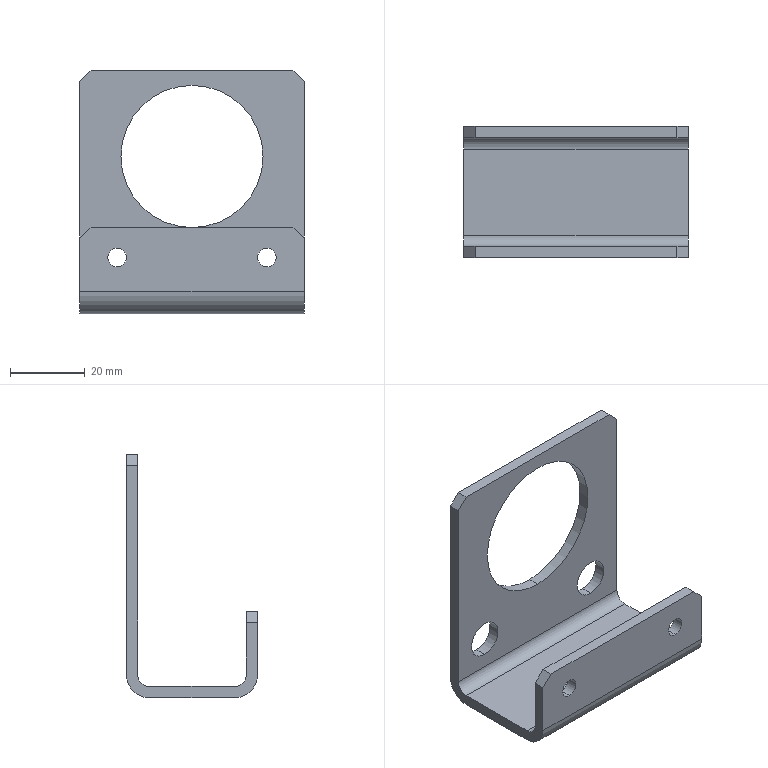Part | SolidWorks | features BaseBody 1 | 1 solid | 28 faces | box 60 x 35 x 65 mm | volume 16319 mm3 | cylinder 14 | plane 14 | commonest cylinder face diameters 5 x4 10 x4 6 x2 12 x2 38 x2
STEP:
#1=CARTESIAN_POINT('',(20.,29.,8.5));
#2=VERTEX_POINT('',#1);
#3=CARTESIAN_POINT('',(20.,29.,-1.5));
#4=VERTEX_POINT('',#3);
#5=CARTESIAN_POINT('',(20.,29.,3.5));
#6=DIRECTION('',(0.,-1.,0.));
#7=DIRECTION('',(0.,0.,-1.));
#8=AXIS2_PLACEMENT_3D('',#5,#6,#7);
#9=CIRCLE('',#8,5.);
#10=EDGE_CURVE('',#2,#4,#9,.T.);
#11=ORIENTED_EDGE('',*,*,#10,.T.);
#12=CARTESIAN_POINT('',(20.,32.,-1.5));
#13=VERTEX_POINT('',#12);
#14=CARTESIAN_POINT('',(20.,22.,-1.5));
#15=DIRECTION('',(0.,1.,0.));
#16=VECTOR('',#15,1000.);
#17=LINE('',#14,#16);
#18=EDGE_CURVE('',#4,#13,#17,.T.);
#19=ORIENTED_EDGE('',*,*,#18,.T.);
#20=CARTESIAN_POINT('',(20.,32.,8.5));
#21=VERTEX_POINT('',#20);
#22=CARTESIAN_POINT('',(20.,32.,3.5));
#23=DIRECTION('',(0.,1.,0.));
#24=DIRECTION('',(0.,0.,1.));
#25=AXIS2_PLACEMENT_3D('',#22,#23,#24);
#26=CIRCLE('',#25,5.);
#27=EDGE_CURVE('',#13,#21,#26,.T.);
#28=ORIENTED_EDGE('',*,*,#27,.T.);
#29=CARTESIAN_POINT('',(20.,22.,8.5));
#30=DIRECTION('',(0.,1.,0.));
#31=VECTOR('',#30,1000.);
#32=LINE('',#29,#31);
#33=EDGE_CURVE('',#2,#21,#32,.T.);
#34=ORIENTED_EDGE('',*,*,#33,.F.);
#35=EDGE_LOOP('',(#11,#19,#28,#34));
#36=FACE_OUTER_BOUND('',#35,.T.);
#37=CARTESIAN_POINT('',(20.,22.,3.5));
#38=DIRECTION('',(0.,1.,0.));
#39=DIRECTION('',(0.,0.,1.));
#40=AXIS2_PLACEMENT_3D('',#37,#38,#39);
#41=CYLINDRICAL_SURFACE('',#40,5.);
#42=ADVANCED_FACE('',(#36),#41,.F.);
#43=CARTESIAN_POINT('',(-20.,29.,8.5));
#44=VERTEX_POINT('',#43);
#45=CARTESIAN_POINT('',(-20.,29.,-1.5));
#46=VERTEX_POINT('',#45);
#47=CARTESIAN_POINT('',(-20.,29.,3.5));
#48=DIRECTION('',(0.,-1.,0.));
#49=DIRECTION('',(0.,0.,-1.));
#50=AXIS2_PLACEMENT_3D('',#47,#48,#49);
#51=CIRCLE('',#50,5.);
#52=EDGE_CURVE('',#44,#46,#51,.T.);
#53=ORIENTED_EDGE('',*,*,#52,.T.);
#54=CARTESIAN_POINT('',(-20.,32.,-1.5));
#55=VERTEX_POINT('',#54);
#56=CARTESIAN_POINT('',(-20.,22.,-1.5));
#57=DIRECTION('',(0.,1.,0.));
#58=VECTOR('',#57,1000.);
#59=LINE('',#56,#58);
#60=EDGE_CURVE('',#46,#55,#59,.T.);
#61=ORIENTED_EDGE('',*,*,#60,.T.);
#62=CARTESIAN_POINT('',(-20.,32.,8.5));
#63=VERTEX_POINT('',#62);
#64=CARTESIAN_POINT('',(-20.,32.,3.5));
#65=DIRECTION('',(0.,1.,0.));
#66=DIRECTION('',(0.,0.,1.));
#67=AXIS2_PLACEMENT_3D('',#64,#65,#66);
#68=CIRCLE('',#67,5.);
#69=EDGE_CURVE('',#55,#63,#68,.T.);
#70=ORIENTED_EDGE('',*,*,#69,.T.);
#71=CARTESIAN_POINT('',(-20.,22.,8.5));
#72=DIRECTION('',(0.,1.,0.));
#73=VECTOR('',#72,1000.);
#74=LINE('',#71,#73);
#75=EDGE_CURVE('',#44,#63,#74,.T.);
#76=ORIENTED_EDGE('',*,*,#75,.F.);
#77=EDGE_LOOP('',(#53,#61,#70,#76));
#78=FACE_OUTER_BOUND('',#77,.T.);
#79=CARTESIAN_POINT('',(-20.,22.,3.5));
#80=DIRECTION('',(0.,1.,0.));
#81=DIRECTION('',(0.,0.,1.));
#82=AXIS2_PLACEMENT_3D('',#79,#80,#81);
#83=CYLINDRICAL_SURFACE('',#82,5.);
#84=ADVANCED_FACE('',(#78),#83,.F.);
#85=CARTESIAN_POINT('',(0.,29.,11.5));
#86=VERTEX_POINT('',#85);
#87=CARTESIAN_POINT('',(0.,29.,49.5));
#88=VERTEX_POINT('',#87);
#89=CARTESIAN_POINT('',(0.,29.,30.5));
#90=DIRECTION('',(0.,1.,0.));
#91=DIRECTION('',(0.,0.,-1.));
#92=AXIS2_PLACEMENT_3D('',#89,#90,#91);
#93=CIRCLE('',#92,19.);
#94=EDGE_CURVE('',#86,#88,#93,.T.);
#95=ORIENTED_EDGE('',*,*,#94,.F.);
#96=CARTESIAN_POINT('',(0.,32.,11.5));
#97=VERTEX_POINT('',#96);
#98=CARTESIAN_POINT('',(0.,-3.001,11.5));
#99=DIRECTION('',(0.,1.,0.));
#100=VECTOR('',#99,1000.);
#101=LINE('',#98,#100);
#102=EDGE_CURVE('',#86,#97,#101,.T.);
#103=ORIENTED_EDGE('',*,*,#102,.T.);
#104=CARTESIAN_POINT('',(0.,32.,49.5));
#105=VERTEX_POINT('',#104);
#106=CARTESIAN_POINT('',(0.,32.,30.5));
#107=DIRECTION('',(0.,1.,0.));
#108=DIRECTION('',(0.,0.,1.));
#109=AXIS2_PLACEMENT_3D('',#106,#107,#108);
#110=CIRCLE('',#109,19.);
#111=EDGE_CURVE('',#97,#105,#110,.T.);
#112=ORIENTED_EDGE('',*,*,#111,.T.);
#113=CARTESIAN_POINT('',(0.,-3.001,49.5));
#114=DIRECTION('',(0.,1.,0.));
#115=VECTOR('',#114,1000.);
#116=LINE('',#113,#115);
#117=EDGE_CURVE('',#88,#105,#116,.T.);
#118=ORIENTED_EDGE('',*,*,#117,.F.);
#119=EDGE_LOOP('',(#95,#103,#112,#118));
#120=FACE_OUTER_BOUND('',#119,.T.);
#121=CARTESIAN_POINT('',(0.,-3.001,30.5));
#122=DIRECTION('',(0.,1.,0.));
#123=DIRECTION('',(0.,0.,1.));
#124=AXIS2_PLACEMENT_3D('',#121,#122,#123);
#125=CYLINDRICAL_SURFACE('',#124,19.);
#126=ADVANCED_FACE('',(#120),#125,.F.);
#127=CARTESIAN_POINT('',(-20.,0.,1.));
#128=VERTEX_POINT('',#127);
#129=CARTESIAN_POINT('',(-20.,0.,6.));
#130=VERTEX_POINT('',#129);
#131=CARTESIAN_POINT('',(-20.,0.,3.5));
#132=DIRECTION('',(0.,1.,0.));
#133=DIRECTION('',(0.,0.,1.));
#134=AXIS2_PLACEMENT_3D('',#131,#132,#133);
#135=CIRCLE('',#134,2.5);
#136=EDGE_CURVE('',#128,#130,#135,.T.);
#137=ORIENTED_EDGE('',*,*,#136,.T.);
#138=CARTESIAN_POINT('',(-20.,-3.,6.));
#139=VERTEX_POINT('',#138);
#140=CARTESIAN_POINT('',(-20.,-3.,6.));
#141=DIRECTION('',(0.,-1.,0.));
#142=VECTOR('',#141,1000.);
#143=LINE('',#140,#142);
#144=EDGE_CURVE('',#130,#139,#143,.T.);
#145=ORIENTED_EDGE('',*,*,#144,.T.);
#146=CARTESIAN_POINT('',(-20.,-3.,1.));
#147=VERTEX_POINT('',#146);
#148=CARTESIAN_POINT('',(-20.,-3.,3.5));
#149=DIRECTION('',(0.,-1.,0.));
#150=DIRECTION('',(0.,0.,-1.));
#151=AXIS2_PLACEMENT_3D('',#148,#149,#150);
#152=CIRCLE('',#151,2.5);
#153=EDGE_CURVE('',#139,#147,#152,.T.);
#154=ORIENTED_EDGE('',*,*,#153,.T.);
#155=CARTESIAN_POINT('',(-20.,-3.,1.));
#156=DIRECTION('',(0.,-1.,0.));
#157=VECTOR('',#156,1000.);
#158=LINE('',#155,#157);
#159=EDGE_CURVE('',#128,#147,#158,.T.);
#160=ORIENTED_EDGE('',*,*,#159,.F.);
#161=EDGE_LOOP('',(#137,#145,#154,#160));
#162=FACE_OUTER_BOUND('',#161,.T.);
#163=CARTESIAN_POINT('',(-20.,-3.,3.5));
#164=DIRECTION('',(0.,-1.,0.));
#165=DIRECTION('',(0.,0.,-1.));
#166=AXIS2_PLACEMENT_3D('',#163,#164,#165);
#167=CYLINDRICAL_SURFACE('',#166,2.5);
#168=ADVANCED_FACE('',(#162),#167,.F.);
#169=CARTESIAN_POINT('',(20.,0.,1.));
#170=VERTEX_POINT('',#169);
#171=CARTESIAN_POINT('',(20.,0.,6.));
#172=VERTEX_POINT('',#171);
#173=CARTESIAN_POINT('',(20.,0.,3.5));
#174=DIRECTION('',(0.,1.,0.));
#175=DIRECTION('',(0.,0.,1.));
#176=AXIS2_PLACEMENT_3D('',#173,#174,#175);
#177=CIRCLE('',#176,2.5);
#178=EDGE_CURVE('',#170,#172,#177,.T.);
#179=ORIENTED_EDGE('',*,*,#178,.T.);
#180=CARTESIAN_POINT('',(20.,-3.,6.));
#181=VERTEX_POINT('',#180);
#182=CARTESIAN_POINT('',(20.,-3.,6.));
#183=DIRECTION('',(0.,-1.,0.));
#184=VECTOR('',#183,1000.);
#185=LINE('',#182,#184);
#186=EDGE_CURVE('',#172,#181,#185,.T.);
#187=ORIENTED_EDGE('',*,*,#186,.T.);
#188=CARTESIAN_POINT('',(20.,-3.,1.));
#189=VERTEX_POINT('',#188);
#190=CARTESIAN_POINT('',(20.,-3.,3.5));
#191=DIRECTION('',(0.,-1.,0.));
#192=DIRECTION('',(0.,0.,-1.));
#193=AXIS2_PLACEMENT_3D('',#190,#191,#192);
#194=CIRCLE('',#193,2.5);
#195=EDGE_CURVE('',#181,#189,#194,.T.);
#196=ORIENTED_EDGE('',*,*,#195,.T.);
#197=CARTESIAN_POINT('',(20.,-3.,1.));
#198=DIRECTION('',(0.,-1.,0.));
#199=VECTOR('',#198,1000.);
#200=LINE('',#197,#199);
#201=EDGE_CURVE('',#170,#189,#200,.T.);
#202=ORIENTED_EDGE('',*,*,#201,.F.);
#203=EDGE_LOOP('',(#179,#187,#196,#202));
#204=FACE_OUTER_BOUND('',#203,.T.);
#205=CARTESIAN_POINT('',(20.,-3.,3.5));
#206=DIRECTION('',(0.,-1.,0.));
#207=DIRECTION('',(0.,0.,-1.));
#208=AXIS2_PLACEMENT_3D('',#205,#206,#207);
#209=CYLINDRICAL_SURFACE('',#208,2.5);
#210=ADVANCED_FACE('',(#204),#209,.F.);
#211=CARTESIAN_POINT('',(27.,32.,53.5));
#212=VERTEX_POINT('',#211);
#213=CARTESIAN_POINT('',(30.,32.,50.5));
#214=VERTEX_POINT('',#213);
#215=CARTESIAN_POINT('',(30.,32.,50.5));
#216=DIRECTION('',(0.7071,0.,-0.7071));
#217=VECTOR('',#216,1000.);
#218=LINE('',#215,#217);
#219=EDGE_CURVE('',#212,#214,#218,.T.);
#220=ORIENTED_EDGE('',*,*,#219,.F.);
#221=CARTESIAN_POINT('',(27.,29.,53.5));
#222=VERTEX_POINT('',#221);
#223=CARTESIAN_POINT('',(27.,32.,53.5));
#224=DIRECTION('',(0.,1.,0.));
#225=VECTOR('',#224,1000.);
#226=LINE('',#223,#225);
#227=EDGE_CURVE('',#222,#212,#226,.T.);
#228=ORIENTED_EDGE('',*,*,#227,.F.);
#229=CARTESIAN_POINT('',(30.,29.,50.5));
#230=VERTEX_POINT('',#229);
#231=CARTESIAN_POINT('',(40.25,29.,40.25));
#232=DIRECTION('',(-0.7071,0.,0.7071));
#233=VECTOR('',#232,1000.);
#234=LINE('',#231,#233);
#235=EDGE_CURVE('',#230,#222,#234,.T.);
#236=ORIENTED_EDGE('',*,*,#235,.F.);
#237=CARTESIAN_POINT('',(30.,32.,50.5));
#238=DIRECTION('',(0.,-1.,0.));
#239=VECTOR('',#238,1000.);
#240=LINE('',#237,#239);
#241=EDGE_CURVE('',#214,#230,#240,.T.);
#242=ORIENTED_EDGE('',*,*,#241,.F.);
#243=EDGE_LOOP('',(#220,#228,#236,#242));
#244=FACE_OUTER_BOUND('',#243,.T.);
#245=CARTESIAN_POINT('',(30.,32.,50.5));
#246=DIRECTION('',(-0.7071,0.,-0.7071));
#247=DIRECTION('',(-0.7071,0.,0.7071));
#248=AXIS2_PLACEMENT_3D('',#245,#246,#247);
#249=PLANE('',#248);
#250=ADVANCED_FACE('',(#244),#249,.F.);
#251=CARTESIAN_POINT('',(-30.,32.,50.5));
#252=VERTEX_POINT('',#251);
#253=CARTESIAN_POINT('',(-27.,32.,53.5));
#254=VERTEX_POINT('',#253);
#255=CARTESIAN_POINT('',(-27.,32.,53.5));
#256=DIRECTION('',(0.7071,0.,0.7071));
#257=VECTOR('',#256,1000.);
#258=LINE('',#255,#257);
#259=EDGE_CURVE('',#252,#254,#258,.T.);
#260=ORIENTED_EDGE('',*,*,#259,.F.);
#261=CARTESIAN_POINT('',(-30.,29.,50.5));
#262=VERTEX_POINT('',#261);
#263=CARTESIAN_POINT('',(-30.,32.,50.5));
#264=DIRECTION('',(0.,1.,0.));
#265=VECTOR('',#264,1000.);
#266=LINE('',#263,#265);
#267=EDGE_CURVE('',#262,#252,#266,.T.);
#268=ORIENTED_EDGE('',*,*,#267,.F.);
#269=CARTESIAN_POINT('',(-27.,29.,53.5));
#270=VERTEX_POINT('',#269);
#271=CARTESIAN_POINT('',(-40.25,29.,40.25));
#272=DIRECTION('',(-0.7071,0.,-0.7071));
#273=VECTOR('',#272,1000.);
#274=LINE('',#271,#273);
#275=EDGE_CURVE('',#270,#262,#274,.T.);
#276=ORIENTED_EDGE('',*,*,#275,.F.);
#277=CARTESIAN_POINT('',(-27.,32.,53.5));
#278=DIRECTION('',(0.,-1.,0.));
#279=VECTOR('',#278,1000.);
#280=LINE('',#277,#279);
#281=EDGE_CURVE('',#254,#270,#280,.T.);
#282=ORIENTED_EDGE('',*,*,#281,.F.);
#283=EDGE_LOOP('',(#260,#268,#276,#282));
#284=FACE_OUTER_BOUND('',#283,.T.);
#285=CARTESIAN_POINT('',(-27.,32.,53.5));
#286=DIRECTION('',(0.7071,0.,-0.7071));
#287=DIRECTION('',(0.,-1.,0.));
#288=AXIS2_PLACEMENT_3D('',#285,#286,#287);
#289=PLANE('',#288);
#290=ADVANCED_FACE('',(#284),#289,.F.);
#291=CARTESIAN_POINT('',(-27.,-3.,11.5));
#292=VERTEX_POINT('',#291);
#293=CARTESIAN_POINT('',(-30.,-3.,8.5));
#294=VERTEX_POINT('',#293);
#295=CARTESIAN_POINT('',(-30.,-3.,8.5));
#296=DIRECTION('',(-0.7071,0.,-0.7071));
#297=VECTOR('',#296,1000.);
#298=LINE('',#295,#297);
#299=EDGE_CURVE('',#292,#294,#298,.T.);
#300=ORIENTED_EDGE('',*,*,#299,.F.);
#301=CARTESIAN_POINT('',(-27.,0.,11.5));
#302=VERTEX_POINT('',#301);
#303=CARTESIAN_POINT('',(-27.,-3.,11.5));
#304=DIRECTION('',(0.,-1.,0.));
#305=VECTOR('',#304,1000.);
#306=LINE('',#303,#305);
#307=EDGE_CURVE('',#302,#292,#306,.T.);
#308=ORIENTED_EDGE('',*,*,#307,.F.);
#309=CARTESIAN_POINT('',(-30.,0.,8.5));
#310=VERTEX_POINT('',#309);
#311=CARTESIAN_POINT('',(-19.25,0.,19.25));
#312=DIRECTION('',(0.7071,0.,0.7071));
#313=VECTOR('',#312,1000.);
#314=LINE('',#311,#313);
#315=EDGE_CURVE('',#310,#302,#314,.T.);
#316=ORIENTED_EDGE('',*,*,#315,.F.);
#317=CARTESIAN_POINT('',(-30.,-3.,8.5));
#318=DIRECTION('',(0.,1.,0.));
#319=VECTOR('',#318,1000.);
#320=LINE('',#317,#319);
#321=EDGE_CURVE('',#294,#310,#320,.T.);
#322=ORIENTED_EDGE('',*,*,#321,.F.);
#323=EDGE_LOOP('',(#300,#308,#316,#322));
#324=FACE_OUTER_BOUND('',#323,.T.);
#325=CARTESIAN_POINT('',(-30.,-3.,8.5));
#326=DIRECTION('',(0.7071,0.,-0.7071));
#327=DIRECTION('',(0.,-1.,0.));
#328=AXIS2_PLACEMENT_3D('',#325,#326,#327);
#329=PLANE('',#328);
#330=ADVANCED_FACE('',(#324),#329,.F.);
#331=CARTESIAN_POINT('',(30.,-3.,8.5));
#332=VERTEX_POINT('',#331);
#333=CARTESIAN_POINT('',(27.,-3.,11.5));
#334=VERTEX_POINT('',#333);
#335=CARTESIAN_POINT('',(27.,-3.,11.5));
#336=DIRECTION('',(-0.7071,0.,0.7071));
#337=VECTOR('',#336,1000.);
#338=LINE('',#335,#337);
#339=EDGE_CURVE('',#332,#334,#338,.T.);
#340=ORIENTED_EDGE('',*,*,#339,.F.);
#341=CARTESIAN_POINT('',(30.,0.,8.5));
#342=VERTEX_POINT('',#341);
#343=CARTESIAN_POINT('',(30.,-3.,8.5));
#344=DIRECTION('',(0.,-1.,0.));
#345=VECTOR('',#344,1000.);
#346=LINE('',#343,#345);
#347=EDGE_CURVE('',#342,#332,#346,.T.);
#348=ORIENTED_EDGE('',*,*,#347,.F.);
#349=CARTESIAN_POINT('',(27.,0.,11.5));
#350=VERTEX_POINT('',#349);
#351=CARTESIAN_POINT('',(19.25,0.,19.25));
#352=DIRECTION('',(0.7071,0.,-0.7071));
#353=VECTOR('',#352,1000.);
#354=LINE('',#351,#353);
#355=EDGE_CURVE('',#350,#342,#354,.T.);
#356=ORIENTED_EDGE('',*,*,#355,.F.);
#357=CARTESIAN_POINT('',(27.,-3.,11.5));
#358=DIRECTION('',(0.,1.,0.));
#359=VECTOR('',#358,1000.);
#360=LINE('',#357,#359);
#361=EDGE_CURVE('',#334,#350,#360,.T.);
#362=ORIENTED_EDGE('',*,*,#361,.F.);
#363=EDGE_LOOP('',(#340,#348,#356,#362));
#364=FACE_OUTER_BOUND('',#363,.T.);
#365=CARTESIAN_POINT('',(27.,-3.,11.5));
#366=DIRECTION('',(-0.7071,0.,-0.7071));
#367=DIRECTION('',(-0.7071,0.,0.7071));
#368=AXIS2_PLACEMENT_3D('',#365,#366,#367);
#369=PLANE('',#368);
#370=ADVANCED_FACE('',(#364),#369,.F.);
#371=CARTESIAN_POINT('',(0.,32.,53.5));
#372=DIRECTION('',(1.,0.,0.));
#373=VECTOR('',#372,1000.);
#374=LINE('',#371,#373);
#375=EDGE_CURVE('',#254,#212,#374,.T.);
#376=ORIENTED_EDGE('',*,*,#375,.F.);
#377=ORIENTED_EDGE('',*,*,#281,.T.);
#378=CARTESIAN_POINT('',(30.,29.,53.5));
#379=DIRECTION('',(1.,0.,0.));
#380=VECTOR('',#379,1000.);
#381=LINE('',#378,#380);
#382=EDGE_CURVE('',#270,#222,#381,.T.);
#383=ORIENTED_EDGE('',*,*,#382,.T.);
#384=ORIENTED_EDGE('',*,*,#227,.T.);
#385=EDGE_LOOP('',(#376,#377,#383,#384));
#386=FACE_OUTER_BOUND('',#385,.T.);
#387=CARTESIAN_POINT('',(30.,32.,53.5));
#388=DIRECTION('',(0.,0.,-1.));
#389=DIRECTION('',(0.,-1.,0.));
#390=AXIS2_PLACEMENT_3D('',#387,#388,#389);
#391=PLANE('',#390);
#392=ADVANCED_FACE('',(#386),#391,.F.);
#393=CARTESIAN_POINT('',(0.,29.,30.5));
#394=DIRECTION('',(0.,1.,0.));
#395=DIRECTION('',(0.,0.,-1.));
#396=AXIS2_PLACEMENT_3D('',#393,#394,#395);
#397=CIRCLE('',#396,19.);
#398=EDGE_CURVE('',#88,#86,#397,.T.);
#399=ORIENTED_EDGE('',*,*,#398,.T.);
#400=ORIENTED_EDGE('',*,*,#94,.T.);
#401=EDGE_LOOP('',(#399,#400));
#402=FACE_BOUND('',#401,.T.);
#403=ORIENTED_EDGE('',*,*,#52,.F.);
#404=CARTESIAN_POINT('',(-20.,29.,3.5));
#405=DIRECTION('',(0.,-1.,0.));
#406=DIRECTION('',(0.,0.,-1.));
#407=AXIS2_PLACEMENT_3D('',#404,#405,#406);
#408=CIRCLE('',#407,5.);
#409=EDGE_CURVE('',#46,#44,#408,.T.);
#410=ORIENTED_EDGE('',*,*,#409,.F.);
#411=EDGE_LOOP('',(#403,#410));
#412=FACE_BOUND('',#411,.T.);
#413=ORIENTED_EDGE('',*,*,#10,.F.);
#414=CARTESIAN_POINT('',(20.,29.,3.5));
#415=DIRECTION('',(0.,-1.,0.));
#416=DIRECTION('',(0.,0.,-1.));
#417=AXIS2_PLACEMENT_3D('',#414,#415,#416);
#418=CIRCLE('',#417,5.);
#419=EDGE_CURVE('',#4,#2,#418,.T.);
#420=ORIENTED_EDGE('',*,*,#419,.F.);
#421=EDGE_LOOP('',(#413,#420));
#422=FACE_BOUND('',#421,.T.);
#423=ORIENTED_EDGE('',*,*,#382,.F.);
#424=ORIENTED_EDGE('',*,*,#275,.T.);
#425=CARTESIAN_POINT('',(-30.,29.,-5.5));
#426=VERTEX_POINT('',#425);
#427=CARTESIAN_POINT('',(-30.,29.,53.5));
#428=DIRECTION('',(0.,0.,1.));
#429=VECTOR('',#428,1000.);
#430=LINE('',#427,#429);
#431=EDGE_CURVE('',#426,#262,#430,.T.);
#432=ORIENTED_EDGE('',*,*,#431,.F.);
#433=CARTESIAN_POINT('',(30.,29.,-5.5));
#434=VERTEX_POINT('',#433);
#435=CARTESIAN_POINT('',(30.,29.,-5.5));
#436=DIRECTION('',(-1.,0.,0.));
#437=VECTOR('',#436,1000.);
#438=LINE('',#435,#437);
#439=EDGE_CURVE('',#434,#426,#438,.T.);
#440=ORIENTED_EDGE('',*,*,#439,.F.);
#441=CARTESIAN_POINT('',(30.,29.,-8.5));
#442=DIRECTION('',(0.,0.,-1.));
#443=VECTOR('',#442,1000.);
#444=LINE('',#441,#443);
#445=EDGE_CURVE('',#230,#434,#444,.T.);
#446=ORIENTED_EDGE('',*,*,#445,.F.);
#447=ORIENTED_EDGE('',*,*,#235,.T.);
#448=EDGE_LOOP('',(#423,#424,#432,#440,#446,#447));
#449=FACE_OUTER_BOUND('',#448,.T.);
#450=CARTESIAN_POINT('',(0.,29.,0.));
#451=DIRECTION('',(0.,-1.,0.));
#452=DIRECTION('',(-1.,0.,0.));
#453=AXIS2_PLACEMENT_3D('',#450,#451,#452);
#454=PLANE('',#453);
#455=ADVANCED_FACE('',(#402,#412,#422,#449),#454,.T.);
#456=CARTESIAN_POINT('',(0.,32.,30.5));
#457=DIRECTION('',(0.,1.,0.));
#458=DIRECTION('',(0.,0.,1.));
#459=AXIS2_PLACEMENT_3D('',#456,#457,#458);
#460=CIRCLE('',#459,19.);
#461=EDGE_CURVE('',#105,#97,#460,.T.);
#462=ORIENTED_EDGE('',*,*,#461,.F.);
#463=ORIENTED_EDGE('',*,*,#111,.F.);
#464=EDGE_LOOP('',(#462,#463));
#465=FACE_BOUND('',#464,.T.);
#466=CARTESIAN_POINT('',(-20.,32.,3.5));
#467=DIRECTION('',(0.,1.,0.));
#468=DIRECTION('',(0.,0.,1.));
#469=AXIS2_PLACEMENT_3D('',#466,#467,#468);
#470=CIRCLE('',#469,5.);
#471=EDGE_CURVE('',#63,#55,#470,.T.);
#472=ORIENTED_EDGE('',*,*,#471,.F.);
#473=ORIENTED_EDGE('',*,*,#69,.F.);
#474=EDGE_LOOP('',(#472,#473));
#475=FACE_BOUND('',#474,.T.);
#476=CARTESIAN_POINT('',(20.,32.,3.5));
#477=DIRECTION('',(0.,1.,0.));
#478=DIRECTION('',(0.,0.,1.));
#479=AXIS2_PLACEMENT_3D('',#476,#477,#478);
#480=CIRCLE('',#479,5.);
#481=EDGE_CURVE('',#21,#13,#480,.T.);
#482=ORIENTED_EDGE('',*,*,#481,.F.);
#483=ORIENTED_EDGE('',*,*,#27,.F.);
#484=EDGE_LOOP('',(#482,#483));
#485=FACE_BOUND('',#484,.T.);
#486=CARTESIAN_POINT('',(-30.,32.,-5.5));
#487=VERTEX_POINT('',#486);
#488=CARTESIAN_POINT('',(-30.,32.,0.));
#489=DIRECTION('',(0.,0.,1.));
#490=VECTOR('',#489,1000.);
#491=LINE('',#488,#490);
#492=EDGE_CURVE('',#487,#252,#491,.T.);
#493=ORIENTED_EDGE('',*,*,#492,.T.);
#494=ORIENTED_EDGE('',*,*,#259,.T.);
#495=ORIENTED_EDGE('',*,*,#375,.T.);
#496=ORIENTED_EDGE('',*,*,#219,.T.);
#497=CARTESIAN_POINT('',(30.,32.,-5.5));
#498=VERTEX_POINT('',#497);
#499=CARTESIAN_POINT('',(30.,32.,0.));
#500=DIRECTION('',(0.,0.,-1.));
#501=VECTOR('',#500,1000.);
#502=LINE('',#499,#501);
#503=EDGE_CURVE('',#214,#498,#502,.T.);
#504=ORIENTED_EDGE('',*,*,#503,.T.);
#505=CARTESIAN_POINT('',(30.,32.,-5.5));
#506=DIRECTION('',(1.,0.,0.));
#507=VECTOR('',#506,1000.);
#508=LINE('',#505,#507);
#509=EDGE_CURVE('',#487,#498,#508,.T.);
#510=ORIENTED_EDGE('',*,*,#509,.F.);
#511=EDGE_LOOP('',(#493,#494,#495,#496,#504,#510));
#512=FACE_OUTER_BOUND('',#511,.T.);
#513=CARTESIAN_POINT('',(0.,32.,0.));
#514=DIRECTION('',(0.,-1.,0.));
#515=DIRECTION('',(-1.,0.,0.));
#516=AXIS2_PLACEMENT_3D('',#513,#514,#515);
#517=PLANE('',#516);
#518=ADVANCED_FACE('',(#465,#475,#485,#512),#517,.F.);
#519=CARTESIAN_POINT('',(-30.,26.,-8.5));
#520=VERTEX_POINT('',#519);
#521=CARTESIAN_POINT('',(30.,26.,-8.5));
#522=VERTEX_POINT('',#521);
#523=CARTESIAN_POINT('',(-30.,26.,-8.5));
#524=DIRECTION('',(1.,0.,0.));
#525=VECTOR('',#524,1000.);
#526=LINE('',#523,#525);
#527=EDGE_CURVE('',#520,#522,#526,.T.);
#528=ORIENTED_EDGE('',*,*,#527,.T.);
#529=CARTESIAN_POINT('',(30.,26.,-5.5));
#530=DIRECTION('',(1.,0.,0.));
#531=DIRECTION('',(0.,0.,1.));
#532=AXIS2_PLACEMENT_3D('',#529,#530,#531);
#533=CIRCLE('',#532,3.);
#534=EDGE_CURVE('',#522,#434,#533,.T.);
#535=ORIENTED_EDGE('',*,*,#534,.T.);
#536=ORIENTED_EDGE('',*,*,#439,.T.);
#537=CARTESIAN_POINT('',(-30.,26.,-5.5));
#538=DIRECTION('',(-1.,0.,0.));
#539=DIRECTION('',(0.,0.,1.));
#540=AXIS2_PLACEMENT_3D('',#537,#538,#539);
#541=CIRCLE('',#540,3.);
#542=EDGE_CURVE('',#426,#520,#541,.T.);
#543=ORIENTED_EDGE('',*,*,#542,.T.);
#544=EDGE_LOOP('',(#528,#535,#536,#543));
#545=FACE_OUTER_BOUND('',#544,.T.);
#546=CARTESIAN_POINT('',(-30.,26.,-5.5));
#547=DIRECTION('',(-1.,0.,0.));
#548=DIRECTION('',(0.,1.,0.));
#549=AXIS2_PLACEMENT_3D('',#546,#547,#548);
#550=CYLINDRICAL_SURFACE('',#549,3.);
#551=ADVANCED_FACE('',(#545),#550,.F.);
#552=CARTESIAN_POINT('',(-30.,26.,-11.5));
#553=VERTEX_POINT('',#552);
#554=CARTESIAN_POINT('',(30.,26.,-11.5));
#555=VERTEX_POINT('',#554);
#556=CARTESIAN_POINT('',(-30.,26.,-11.5));
#557=DIRECTION('',(1.,0.,0.));
#558=VECTOR('',#557,1000.);
#559=LINE('',#556,#558);
#560=EDGE_CURVE('',#553,#555,#559,.T.);
#561=ORIENTED_EDGE('',*,*,#560,.F.);
#562=CARTESIAN_POINT('',(-30.,26.,-5.5));
#563=DIRECTION('',(-1.,0.,0.));
#564=DIRECTION('',(0.,0.,1.));
#565=AXIS2_PLACEMENT_3D('',#562,#563,#564);
#566=CIRCLE('',#565,6.);
#567=EDGE_CURVE('',#487,#553,#566,.T.);
#568=ORIENTED_EDGE('',*,*,#567,.F.);
#569=ORIENTED_EDGE('',*,*,#509,.T.);
#570=CARTESIAN_POINT('',(30.,26.,-5.5));
#571=DIRECTION('',(1.,0.,0.));
#572=DIRECTION('',(0.,0.,1.));
#573=AXIS2_PLACEMENT_3D('',#570,#571,#572);
#574=CIRCLE('',#573,6.);
#575=EDGE_CURVE('',#555,#498,#574,.T.);
#576=ORIENTED_EDGE('',*,*,#575,.F.);
#577=EDGE_LOOP('',(#561,#568,#569,#576));
#578=FACE_OUTER_BOUND('',#577,.T.);
#579=CARTESIAN_POINT('',(-30.,26.,-5.5));
#580=DIRECTION('',(-1.,0.,0.));
#581=DIRECTION('',(0.,1.,0.));
#582=AXIS2_PLACEMENT_3D('',#579,#580,#581);
#583=CYLINDRICAL_SURFACE('',#582,6.);
#584=ADVANCED_FACE('',(#578),#583,.T.);
#585=CARTESIAN_POINT('',(-30.,0.,-5.5));
#586=VERTEX_POINT('',#585);
#587=CARTESIAN_POINT('',(30.,0.,-5.5));
#588=VERTEX_POINT('',#587);
#589=CARTESIAN_POINT('',(-30.,0.,-5.5));
#590=DIRECTION('',(1.,0.,0.));
#591=VECTOR('',#590,1000.);
#592=LINE('',#589,#591);
#593=EDGE_CURVE('',#586,#588,#592,.T.);
#594=ORIENTED_EDGE('',*,*,#593,.T.);
#595=CARTESIAN_POINT('',(30.,3.,-8.5));
#596=VERTEX_POINT('',#595);
#597=CARTESIAN_POINT('',(30.,3.,-5.5));
#598=DIRECTION('',(1.,0.,0.));
#599=DIRECTION('',(0.,-1.,0.));
#600=AXIS2_PLACEMENT_3D('',#597,#598,#599);
#601=CIRCLE('',#600,3.);
#602=EDGE_CURVE('',#588,#596,#601,.T.);
#603=ORIENTED_EDGE('',*,*,#602,.T.);
#604=CARTESIAN_POINT('',(-30.,3.,-8.5));
#605=VERTEX_POINT('',#604);
#606=CARTESIAN_POINT('',(30.,3.,-8.5));
#607=DIRECTION('',(-1.,0.,0.));
#608=VECTOR('',#607,1000.);
#609=LINE('',#606,#608);
#610=EDGE_CURVE('',#596,#605,#609,.T.);
#611=ORIENTED_EDGE('',*,*,#610,.T.);
#612=CARTESIAN_POINT('',(-30.,3.,-5.5));
#613=DIRECTION('',(-1.,0.,0.));
#614=DIRECTION('',(0.,-1.,0.));
#615=AXIS2_PLACEMENT_3D('',#612,#613,#614);
#616=CIRCLE('',#615,3.);
#617=EDGE_CURVE('',#605,#586,#616,.T.);
#618=ORIENTED_EDGE('',*,*,#617,.T.);
#619=EDGE_LOOP('',(#594,#603,#611,#618));
#620=FACE_OUTER_BOUND('',#619,.T.);
#621=CARTESIAN_POINT('',(-30.,3.,-5.5));
#622=DIRECTION('',(-1.,0.,0.));
#623=DIRECTION('',(0.,0.,-1.));
#624=AXIS2_PLACEMENT_3D('',#621,#622,#623);
#625=CYLINDRICAL_SURFACE('',#624,3.);
#626=ADVANCED_FACE('',(#620),#625,.F.);
#627=CARTESIAN_POINT('',(-30.,-3.,-5.5));
#628=VERTEX_POINT('',#627);
#629=CARTESIAN_POINT('',(30.,-3.,-5.5));
#630=VERTEX_POINT('',#629);
#631=CARTESIAN_POINT('',(-30.,-3.,-5.5));
#632=DIRECTION('',(1.,0.,0.));
#633=VECTOR('',#632,1000.);
#634=LINE('',#631,#633);
#635=EDGE_CURVE('',#628,#630,#634,.T.);
#636=ORIENTED_EDGE('',*,*,#635,.F.);
#637=CARTESIAN_POINT('',(-30.,3.,-11.5));
#638=VERTEX_POINT('',#637);
#639=CARTESIAN_POINT('',(-30.,3.,-5.5));
#640=DIRECTION('',(-1.,0.,0.));
#641=DIRECTION('',(0.,-1.,0.));
#642=AXIS2_PLACEMENT_3D('',#639,#640,#641);
#643=CIRCLE('',#642,6.);
#644=EDGE_CURVE('',#638,#628,#643,.T.);
#645=ORIENTED_EDGE('',*,*,#644,.F.);
#646=CARTESIAN_POINT('',(30.,3.,-11.5));
#647=VERTEX_POINT('',#646);
#648=CARTESIAN_POINT('',(30.,3.,-11.5));
#649=DIRECTION('',(1.,0.,0.));
#650=VECTOR('',#649,1000.);
#651=LINE('',#648,#650);
#652=EDGE_CURVE('',#638,#647,#651,.T.);
#653=ORIENTED_EDGE('',*,*,#652,.T.);
#654=CARTESIAN_POINT('',(30.,3.,-5.5));
#655=DIRECTION('',(1.,0.,0.));
#656=DIRECTION('',(0.,-1.,0.));
#657=AXIS2_PLACEMENT_3D('',#654,#655,#656);
#658=CIRCLE('',#657,6.);
#659=EDGE_CURVE('',#630,#647,#658,.T.);
#660=ORIENTED_EDGE('',*,*,#659,.F.);
#661=EDGE_LOOP('',(#636,#645,#653,#660));
#662=FACE_OUTER_BOUND('',#661,.T.);
#663=CARTESIAN_POINT('',(-30.,3.,-5.5));
#664=DIRECTION('',(-1.,0.,0.));
#665=DIRECTION('',(0.,0.,-1.));
#666=AXIS2_PLACEMENT_3D('',#663,#664,#665);
#667=CYLINDRICAL_SURFACE('',#666,6.);
#668=ADVANCED_FACE('',(#662),#667,.T.);
#669=CARTESIAN_POINT('',(-30.,-3.,11.5));
#670=DIRECTION('',(1.,0.,0.));
#671=VECTOR('',#670,1000.);
#672=LINE('',#669,#671);
#673=EDGE_CURVE('',#292,#334,#672,.T.);
#674=ORIENTED_EDGE('',*,*,#673,.T.);
#675=ORIENTED_EDGE('',*,*,#361,.T.);
#676=CARTESIAN_POINT('',(-30.,0.,11.5));
#677=DIRECTION('',(1.,0.,0.));
#678=VECTOR('',#677,1000.);
#679=LINE('',#676,#678);
#680=EDGE_CURVE('',#302,#350,#679,.T.);
#681=ORIENTED_EDGE('',*,*,#680,.F.);
#682=ORIENTED_EDGE('',*,*,#307,.T.);
#683=EDGE_LOOP('',(#674,#675,#681,#682));
#684=FACE_OUTER_BOUND('',#683,.T.);
#685=CARTESIAN_POINT('',(-30.,-3.,11.5));
#686=DIRECTION('',(0.,0.,1.));
#687=DIRECTION('',(1.,0.,0.));
#688=AXIS2_PLACEMENT_3D('',#685,#686,#687);
#689=PLANE('',#688);
#690=ADVANCED_FACE('',(#684),#689,.T.);
#691=ORIENTED_EDGE('',*,*,#178,.F.);
#692=CARTESIAN_POINT('',(20.,0.,3.5));
#693=DIRECTION('',(0.,1.,0.));
#694=DIRECTION('',(0.,0.,1.));
#695=AXIS2_PLACEMENT_3D('',#692,#693,#694);
#696=CIRCLE('',#695,2.5);
#697=EDGE_CURVE('',#172,#170,#696,.T.);
#698=ORIENTED_EDGE('',*,*,#697,.F.);
#699=EDGE_LOOP('',(#691,#698));
#700=FACE_BOUND('',#699,.T.);
#701=ORIENTED_EDGE('',*,*,#136,.F.);
#702=CARTESIAN_POINT('',(-20.,0.,3.5));
#703=DIRECTION('',(0.,1.,0.));
#704=DIRECTION('',(0.,0.,1.));
#705=AXIS2_PLACEMENT_3D('',#702,#703,#704);
#706=CIRCLE('',#705,2.5);
#707=EDGE_CURVE('',#130,#128,#706,.T.);
#708=ORIENTED_EDGE('',*,*,#707,.F.);
#709=EDGE_LOOP('',(#701,#708));
#710=FACE_BOUND('',#709,.T.);
#711=ORIENTED_EDGE('',*,*,#680,.T.);
#712=ORIENTED_EDGE('',*,*,#355,.T.);
#713=CARTESIAN_POINT('',(30.,0.,-11.5));
#714=DIRECTION('',(0.,0.,-1.));
#715=VECTOR('',#714,1000.);
#716=LINE('',#713,#715);
#717=EDGE_CURVE('',#342,#588,#716,.T.);
#718=ORIENTED_EDGE('',*,*,#717,.T.);
#719=ORIENTED_EDGE('',*,*,#593,.F.);
#720=CARTESIAN_POINT('',(-30.,0.,-11.5));
#721=DIRECTION('',(0.,0.,1.));
#722=VECTOR('',#721,1000.);
#723=LINE('',#720,#722);
#724=EDGE_CURVE('',#586,#310,#723,.T.);
#725=ORIENTED_EDGE('',*,*,#724,.T.);
#726=ORIENTED_EDGE('',*,*,#315,.T.);
#727=EDGE_LOOP('',(#711,#712,#718,#719,#725,#726));
#728=FACE_OUTER_BOUND('',#727,.T.);
#729=CARTESIAN_POINT('',(0.,0.,0.));
#730=DIRECTION('',(0.,1.,0.));
#731=DIRECTION('',(1.,0.,0.));
#732=AXIS2_PLACEMENT_3D('',#729,#730,#731);
#733=PLANE('',#732);
#734=ADVANCED_FACE('',(#700,#710,#728),#733,.T.);
#735=CARTESIAN_POINT('',(20.,-3.,3.5));
#736=DIRECTION('',(0.,-1.,0.));
#737=DIRECTION('',(0.,0.,-1.));
#738=AXIS2_PLACEMENT_3D('',#735,#736,#737);
#739=CIRCLE('',#738,2.5);
#740=EDGE_CURVE('',#189,#181,#739,.T.);
#741=ORIENTED_EDGE('',*,*,#740,.F.);
#742=ORIENTED_EDGE('',*,*,#195,.F.);
#743=EDGE_LOOP('',(#741,#742));
#744=FACE_BOUND('',#743,.T.);
#745=CARTESIAN_POINT('',(-20.,-3.,3.5));
#746=DIRECTION('',(0.,-1.,0.));
#747=DIRECTION('',(0.,0.,-1.));
#748=AXIS2_PLACEMENT_3D('',#745,#746,#747);
#749=CIRCLE('',#748,2.5);
#750=EDGE_CURVE('',#147,#139,#749,.T.);
#751=ORIENTED_EDGE('',*,*,#750,.F.);
#752=ORIENTED_EDGE('',*,*,#153,.F.);
#753=EDGE_LOOP('',(#751,#752));
#754=FACE_BOUND('',#753,.T.);
#755=CARTESIAN_POINT('',(30.,-3.,-11.5));
#756=DIRECTION('',(0.,0.,-1.));
#757=VECTOR('',#756,1000.);
#758=LINE('',#755,#757);
#759=EDGE_CURVE('',#332,#630,#758,.T.);
#760=ORIENTED_EDGE('',*,*,#759,.F.);
#761=ORIENTED_EDGE('',*,*,#339,.T.);
#762=ORIENTED_EDGE('',*,*,#673,.F.);
#763=ORIENTED_EDGE('',*,*,#299,.T.);
#764=CARTESIAN_POINT('',(-30.,-3.,-11.5));
#765=DIRECTION('',(0.,0.,1.));
#766=VECTOR('',#765,1000.);
#767=LINE('',#764,#766);
#768=EDGE_CURVE('',#628,#294,#767,.T.);
#769=ORIENTED_EDGE('',*,*,#768,.F.);
#770=ORIENTED_EDGE('',*,*,#635,.T.);
#771=EDGE_LOOP('',(#760,#761,#762,#763,#769,#770));
#772=FACE_OUTER_BOUND('',#771,.T.);
#773=CARTESIAN_POINT('',(0.,-3.,0.));
#774=DIRECTION('',(0.,1.,0.));
#775=DIRECTION('',(1.,0.,0.));
#776=AXIS2_PLACEMENT_3D('',#773,#774,#775);
#777=PLANE('',#776);
#778=ADVANCED_FACE('',(#744,#754,#772),#777,.F.);
#779=CARTESIAN_POINT('',(30.,0.,-8.5));
#780=DIRECTION('',(0.,-1.,0.));
#781=VECTOR('',#780,1000.);
#782=LINE('',#779,#781);
#783=EDGE_CURVE('',#522,#596,#782,.T.);
#784=ORIENTED_EDGE('',*,*,#783,.F.);
#785=ORIENTED_EDGE('',*,*,#527,.F.);
#786=CARTESIAN_POINT('',(-30.,32.,-8.5));
#787=DIRECTION('',(0.,1.,0.));
#788=VECTOR('',#787,1000.);
#789=LINE('',#786,#788);
#790=EDGE_CURVE('',#605,#520,#789,.T.);
#791=ORIENTED_EDGE('',*,*,#790,.F.);
#792=ORIENTED_EDGE('',*,*,#610,.F.);
#793=EDGE_LOOP('',(#784,#785,#791,#792));
#794=FACE_OUTER_BOUND('',#793,.T.);
#795=CARTESIAN_POINT('',(0.,0.,-8.5));
#796=DIRECTION('',(0.,0.,1.));
#797=DIRECTION('',(0.,-1.,0.));
#798=AXIS2_PLACEMENT_3D('',#795,#796,#797);
#799=PLANE('',#798);
#800=ADVANCED_FACE('',(#794),#799,.T.);
#801=ORIENTED_EDGE('',*,*,#560,.T.);
#802=CARTESIAN_POINT('',(30.,0.,-11.5));
#803=DIRECTION('',(0.,-1.,0.));
#804=VECTOR('',#803,1000.);
#805=LINE('',#802,#804);
#806=EDGE_CURVE('',#555,#647,#805,.T.);
#807=ORIENTED_EDGE('',*,*,#806,.T.);
#808=ORIENTED_EDGE('',*,*,#652,.F.);
#809=CARTESIAN_POINT('',(-30.,0.,-11.5));
#810=DIRECTION('',(0.,1.,0.));
#811=VECTOR('',#810,1000.);
#812=LINE('',#809,#811);
#813=EDGE_CURVE('',#638,#553,#812,.T.);
#814=ORIENTED_EDGE('',*,*,#813,.T.);
#815=EDGE_LOOP('',(#801,#807,#808,#814));
#816=FACE_OUTER_BOUND('',#815,.T.);
#817=CARTESIAN_POINT('',(0.,0.,-11.5));
#818=DIRECTION('',(0.,0.,1.));
#819=DIRECTION('',(0.,-1.,0.));
#820=AXIS2_PLACEMENT_3D('',#817,#818,#819);
#821=PLANE('',#820);
#822=ADVANCED_FACE('',(#816),#821,.F.);
#823=ORIENTED_EDGE('',*,*,#790,.T.);
#824=ORIENTED_EDGE('',*,*,#542,.F.);
#825=ORIENTED_EDGE('',*,*,#431,.T.);
#826=ORIENTED_EDGE('',*,*,#267,.T.);
#827=ORIENTED_EDGE('',*,*,#492,.F.);
#828=ORIENTED_EDGE('',*,*,#567,.T.);
#829=ORIENTED_EDGE('',*,*,#813,.F.);
#830=ORIENTED_EDGE('',*,*,#644,.T.);
#831=ORIENTED_EDGE('',*,*,#768,.T.);
#832=ORIENTED_EDGE('',*,*,#321,.T.);
#833=ORIENTED_EDGE('',*,*,#724,.F.);
#834=ORIENTED_EDGE('',*,*,#617,.F.);
#835=EDGE_LOOP('',(#823,#824,#825,#826,#827,#828,#829,#830,#831,#832,#833,#834));
#836=FACE_OUTER_BOUND('',#835,.T.);
#837=CARTESIAN_POINT('',(-30.,32.,-11.5));
#838=DIRECTION('',(1.,0.,0.));
#839=DIRECTION('',(0.,-1.,0.));
#840=AXIS2_PLACEMENT_3D('',#837,#838,#839);
#841=PLANE('',#840);
#842=ADVANCED_FACE('',(#836),#841,.F.);
#843=ORIENTED_EDGE('',*,*,#806,.F.);
#844=ORIENTED_EDGE('',*,*,#575,.T.);
#845=ORIENTED_EDGE('',*,*,#503,.F.);
#846=ORIENTED_EDGE('',*,*,#241,.T.);
#847=ORIENTED_EDGE('',*,*,#445,.T.);
#848=ORIENTED_EDGE('',*,*,#534,.F.);
#849=ORIENTED_EDGE('',*,*,#783,.T.);
#850=ORIENTED_EDGE('',*,*,#602,.F.);
#851=ORIENTED_EDGE('',*,*,#717,.F.);
#852=ORIENTED_EDGE('',*,*,#347,.T.);
#853=ORIENTED_EDGE('',*,*,#759,.T.);
#854=ORIENTED_EDGE('',*,*,#659,.T.);
#855=EDGE_LOOP('',(#843,#844,#845,#846,#847,#848,#849,#850,#851,#852,#853,#854));
#856=FACE_OUTER_BOUND('',#855,.T.);
#857=CARTESIAN_POINT('',(30.,0.,-11.5));
#858=DIRECTION('',(-1.,0.,0.));
#859=DIRECTION('',(0.,1.,0.));
#860=AXIS2_PLACEMENT_3D('',#857,#858,#859);
#861=PLANE('',#860);
#862=ADVANCED_FACE('',(#856),#861,.F.);
#863=ORIENTED_EDGE('',*,*,#186,.F.);
#864=ORIENTED_EDGE('',*,*,#697,.T.);
#865=ORIENTED_EDGE('',*,*,#201,.T.);
#866=ORIENTED_EDGE('',*,*,#740,.T.);
#867=EDGE_LOOP('',(#863,#864,#865,#866));
#868=FACE_OUTER_BOUND('',#867,.T.);
#869=CARTESIAN_POINT('',(20.,-3.,3.5));
#870=DIRECTION('',(0.,-1.,0.));
#871=DIRECTION('',(0.,0.,-1.));
#872=AXIS2_PLACEMENT_3D('',#869,#870,#871);
#873=CYLINDRICAL_SURFACE('',#872,2.5);
#874=ADVANCED_FACE('',(#868),#873,.F.);
#875=ORIENTED_EDGE('',*,*,#144,.F.);
#876=ORIENTED_EDGE('',*,*,#707,.T.);
#877=ORIENTED_EDGE('',*,*,#159,.T.);
#878=ORIENTED_EDGE('',*,*,#750,.T.);
#879=EDGE_LOOP('',(#875,#876,#877,#878));
#880=FACE_OUTER_BOUND('',#879,.T.);
#881=CARTESIAN_POINT('',(-20.,-3.,3.5));
#882=DIRECTION('',(0.,-1.,0.));
#883=DIRECTION('',(0.,0.,-1.));
#884=AXIS2_PLACEMENT_3D('',#881,#882,#883);
#885=CYLINDRICAL_SURFACE('',#884,2.5);
#886=ADVANCED_FACE('',(#880),#885,.F.);
#887=ORIENTED_EDGE('',*,*,#102,.F.);
#888=ORIENTED_EDGE('',*,*,#398,.F.);
#889=ORIENTED_EDGE('',*,*,#117,.T.);
#890=ORIENTED_EDGE('',*,*,#461,.T.);
#891=EDGE_LOOP('',(#887,#888,#889,#890));
#892=FACE_OUTER_BOUND('',#891,.T.);
#893=CARTESIAN_POINT('',(0.,-3.001,30.5));
#894=DIRECTION('',(0.,1.,0.));
#895=DIRECTION('',(0.,0.,1.));
#896=AXIS2_PLACEMENT_3D('',#893,#894,#895);
#897=CYLINDRICAL_SURFACE('',#896,19.);
#898=ADVANCED_FACE('',(#892),#897,.F.);
#899=ORIENTED_EDGE('',*,*,#60,.F.);
#900=ORIENTED_EDGE('',*,*,#409,.T.);
#901=ORIENTED_EDGE('',*,*,#75,.T.);
#902=ORIENTED_EDGE('',*,*,#471,.T.);
#903=EDGE_LOOP('',(#899,#900,#901,#902));
#904=FACE_OUTER_BOUND('',#903,.T.);
#905=CARTESIAN_POINT('',(-20.,22.,3.5));
#906=DIRECTION('',(0.,1.,0.));
#907=DIRECTION('',(0.,0.,1.));
#908=AXIS2_PLACEMENT_3D('',#905,#906,#907);
#909=CYLINDRICAL_SURFACE('',#908,5.);
#910=ADVANCED_FACE('',(#904),#909,.F.);
#911=ORIENTED_EDGE('',*,*,#18,.F.);
#912=ORIENTED_EDGE('',*,*,#419,.T.);
#913=ORIENTED_EDGE('',*,*,#33,.T.);
#914=ORIENTED_EDGE('',*,*,#481,.T.);
#915=EDGE_LOOP('',(#911,#912,#913,#914));
#916=FACE_OUTER_BOUND('',#915,.T.);
#917=CARTESIAN_POINT('',(20.,22.,3.5));
#918=DIRECTION('',(0.,1.,0.));
#919=DIRECTION('',(0.,0.,1.));
#920=AXIS2_PLACEMENT_3D('',#917,#918,#919);
#921=CYLINDRICAL_SURFACE('',#920,5.);
#922=ADVANCED_FACE('',(#916),#921,.F.);
#923=CLOSED_SHELL('',(#42,#84,#126,#168,#210,#250,#290,#330,#370,#392,#455,#518,#551,#584,#626,#668,#690,#734,#778,#800,#822,#842,#862,#874,#886,#898,#910,#922));
#924=MANIFOLD_SOLID_BREP('',#923);
#925=CARTESIAN_POINT('',(0.,0.,0.));
#926=DIRECTION('',(0.,0.,1.));
#927=DIRECTION('',(1.,0.,0.));
#928=AXIS2_PLACEMENT_3D('',#925,#926,#927);
#929=(LENGTH_UNIT()NAMED_UNIT(*)SI_UNIT(.MILLI.,.METRE.));
#930=UNCERTAINTY_MEASURE_WITH_UNIT(LENGTH_MEASURE(0.00001),#929,'','');
#931=(NAMED_UNIT(*)PLANE_ANGLE_UNIT()SI_UNIT($,.RADIAN.));
#932=(NAMED_UNIT(*)SI_UNIT($,.STERADIAN.)SOLID_ANGLE_UNIT());
#933=(GEOMETRIC_REPRESENTATION_CONTEXT(3)GLOBAL_UNCERTAINTY_ASSIGNED_CONTEXT((#930))GLOBAL_UNIT_ASSIGNED_CONTEXT((#929,#931,#932))REPRESENTATION_CONTEXT('',''));
#934=ADVANCED_BREP_SHAPE_REPRESENTATION('',(#924,#928),#933);